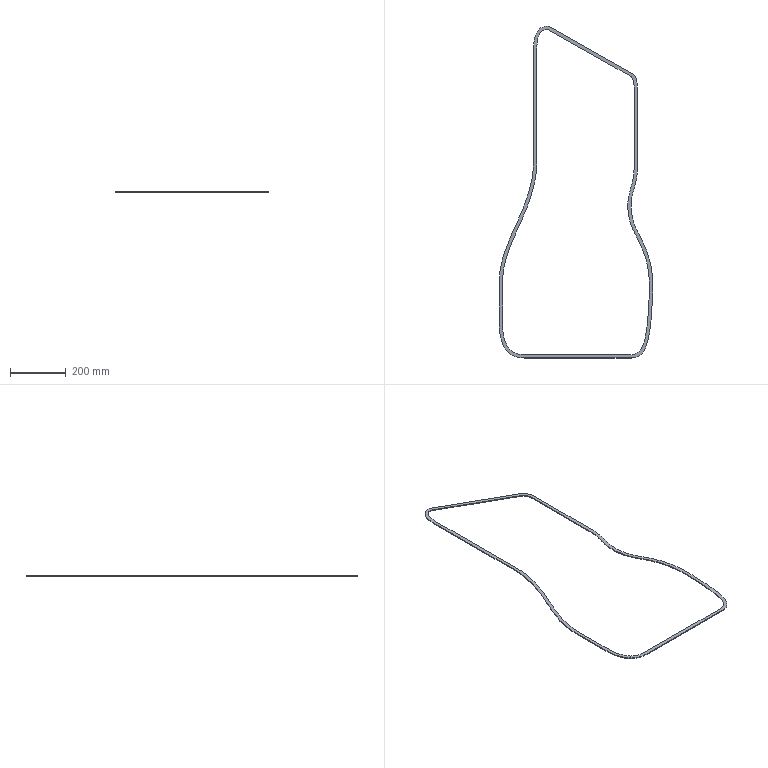Part | SolidWorks | features Extrusion 1 | 1 solid | 229 faces | box 552.5 x 1195 x 3 mm | volume 110448 mm3 | plane 229